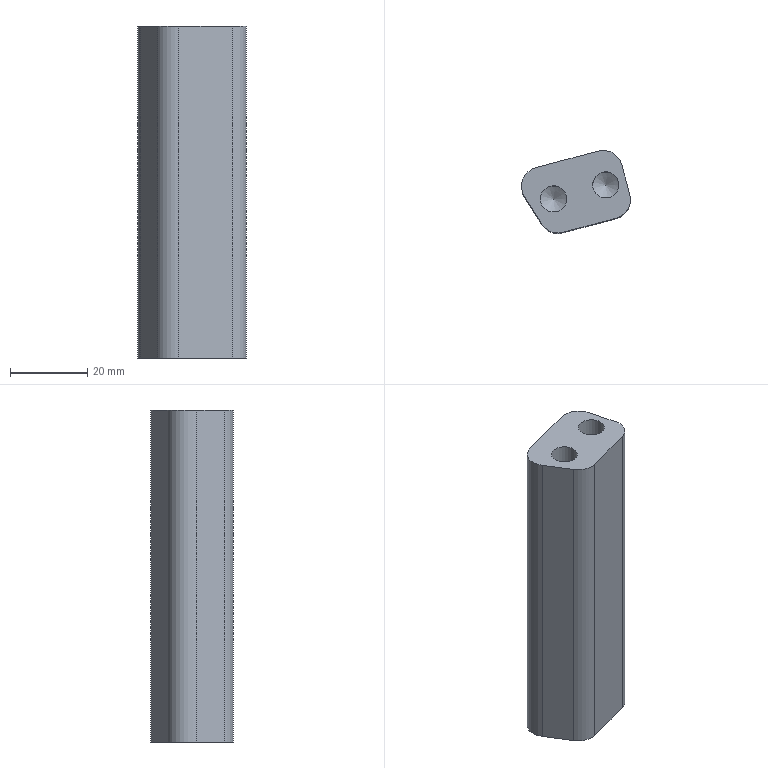Part | NX | features solid 2 | 1 solid | 14 faces | box 28.217 x 21.421 x 86 mm | volume 35584 mm3 | cylinder 6 | plane 6 | cone 2 | commonest cylinder face diameters 10 x4 6.8 x2
STEP:
#1=CARTESIAN_POINT('',(1387.735,54.431,48.508));
#2=VERTEX_POINT('',#1);
#3=CARTESIAN_POINT('',(1384.335,54.431,48.508));
#4=DIRECTION('',(0.,0.,-1.));
#5=DIRECTION('',(1.,0.,0.));
#6=AXIS2_PLACEMENT_3D('',#3,#4,#5);
#7=CIRCLE('',#6,3.4);
#8=EDGE_CURVE('',#2,#2,#7,.F.);
#9=ORIENTED_EDGE('',*,*,#8,.T.);
#10=EDGE_LOOP('',(#9));
#11=FACE_BOUND('',#10,.T.);
#12=CARTESIAN_POINT('',(1384.335,54.431,46.465));
#13=VERTEX_POINT('',#12);
#14=VERTEX_LOOP('',#13);
#15=FACE_BOUND('',#14,.T.);
#16=CARTESIAN_POINT('',(1384.335,54.431,49.018));
#17=DIRECTION('',(0.,0.,1.));
#18=DIRECTION('',(1.,0.,0.));
#19=AXIS2_PLACEMENT_3D('',#16,#17,#18);
#20=CONICAL_SURFACE('',#19,4.25,1.03);
#21=ADVANCED_FACE('',(#11,#15),#20,.F.);
#22=ORIENTED_EDGE('',*,*,#8,.F.);
#23=EDGE_LOOP('',(#22));
#24=FACE_BOUND('',#23,.T.);
#25=CARTESIAN_POINT('',(1380.935,54.431,78.));
#26=VERTEX_POINT('',#25);
#27=CARTESIAN_POINT('',(1384.335,54.431,78.));
#28=DIRECTION('',(0.,0.,1.));
#29=DIRECTION('',(-1.,0.,0.));
#30=AXIS2_PLACEMENT_3D('',#27,#28,#29);
#31=CIRCLE('',#30,3.4);
#32=EDGE_CURVE('',#26,#26,#31,.T.);
#33=ORIENTED_EDGE('',*,*,#32,.T.);
#34=EDGE_LOOP('',(#33));
#35=FACE_BOUND('',#34,.T.);
#36=CARTESIAN_POINT('',(1384.335,54.431,79.018));
#37=DIRECTION('',(0.,0.,-1.));
#38=DIRECTION('',(-1.,0.,0.));
#39=AXIS2_PLACEMENT_3D('',#36,#37,#38);
#40=CYLINDRICAL_SURFACE('',#39,3.4);
#41=ADVANCED_FACE('',(#24,#35),#40,.F.);
#42=CARTESIAN_POINT('',(1366.205,58.89,-8.));
#43=VERTEX_POINT('',#42);
#44=CARTESIAN_POINT('',(1382.352,63.217,-8.));
#45=VERTEX_POINT('',#44);
#46=CARTESIAN_POINT('',(1366.205,58.89,-8.));
#47=DIRECTION('',(0.9659,0.2588,0.));
#48=VECTOR('',#47,1000.);
#49=LINE('',#46,#48);
#50=EDGE_CURVE('',#43,#45,#49,.T.);
#51=ORIENTED_EDGE('',*,*,#50,.T.);
#52=CARTESIAN_POINT('',(1388.475,59.681,-8.));
#53=VERTEX_POINT('',#52);
#54=CARTESIAN_POINT('',(1383.646,58.387,-8.));
#55=DIRECTION('',(0.,0.,-1.));
#56=DIRECTION('',(-1.,0.,0.));
#57=AXIS2_PLACEMENT_3D('',#54,#55,#56);
#58=CIRCLE('',#57,5.);
#59=EDGE_CURVE('',#45,#53,#58,.T.);
#60=ORIENTED_EDGE('',*,*,#59,.T.);
#61=CARTESIAN_POINT('',(1390.546,51.954,-8.));
#62=VERTEX_POINT('',#61);
#63=CARTESIAN_POINT('',(1388.475,59.681,-8.));
#64=DIRECTION('',(0.2588,-0.9659,0.));
#65=VECTOR('',#64,1000.);
#66=LINE('',#63,#65);
#67=EDGE_CURVE('',#53,#62,#66,.T.);
#68=ORIENTED_EDGE('',*,*,#67,.T.);
#69=CARTESIAN_POINT('',(1387.01,45.83,-8.));
#70=VERTEX_POINT('',#69);
#71=CARTESIAN_POINT('',(1385.716,50.66,-8.));
#72=DIRECTION('',(0.,0.,-1.));
#73=DIRECTION('',(-1.,0.,0.));
#74=AXIS2_PLACEMENT_3D('',#71,#72,#73);
#75=CIRCLE('',#74,5.);
#76=EDGE_CURVE('',#62,#70,#75,.T.);
#77=ORIENTED_EDGE('',*,*,#76,.T.);
#78=CARTESIAN_POINT('',(1373.226,42.137,-8.));
#79=VERTEX_POINT('',#78);
#80=CARTESIAN_POINT('',(1387.01,45.83,-8.));
#81=DIRECTION('',(-0.9659,-0.2588,0.));
#82=VECTOR('',#81,1000.);
#83=LINE('',#80,#82);
#84=EDGE_CURVE('',#70,#79,#83,.T.);
#85=ORIENTED_EDGE('',*,*,#84,.T.);
#86=CARTESIAN_POINT('',(1367.692,44.317,-8.));
#87=VERTEX_POINT('',#86);
#88=CARTESIAN_POINT('',(1371.932,46.966,-8.));
#89=DIRECTION('',(0.,0.,-1.));
#90=DIRECTION('',(-1.,0.,0.));
#91=AXIS2_PLACEMENT_3D('',#88,#89,#90);
#92=CIRCLE('',#91,5.);
#93=EDGE_CURVE('',#79,#87,#92,.T.);
#94=ORIENTED_EDGE('',*,*,#93,.T.);
#95=CARTESIAN_POINT('',(1363.259,51.411,-8.));
#96=VERTEX_POINT('',#95);
#97=CARTESIAN_POINT('',(1367.692,44.317,-8.));
#98=DIRECTION('',(-0.5299,0.848,0.));
#99=VECTOR('',#98,1000.);
#100=LINE('',#97,#99);
#101=EDGE_CURVE('',#87,#96,#100,.T.);
#102=ORIENTED_EDGE('',*,*,#101,.T.);
#103=CARTESIAN_POINT('',(1367.499,54.061,-8.));
#104=DIRECTION('',(0.,0.,-1.));
#105=DIRECTION('',(-1.,0.,0.));
#106=AXIS2_PLACEMENT_3D('',#103,#104,#105);
#107=CIRCLE('',#106,5.);
#108=EDGE_CURVE('',#96,#43,#107,.T.);
#109=ORIENTED_EDGE('',*,*,#108,.T.);
#110=EDGE_LOOP('',(#51,#60,#68,#77,#85,#94,#102,#109));
#111=FACE_BOUND('',#110,.T.);
#112=CARTESIAN_POINT('',(1383.646,58.387,-8.));
#113=DIRECTION('',(0.,0.,-1.));
#114=DIRECTION('',(-1.,0.,0.));
#115=AXIS2_PLACEMENT_3D('',#112,#113,#114);
#116=PLANE('',#115);
#117=ADVANCED_FACE('',(#111),#116,.T.);
#118=CARTESIAN_POINT('',(1374.212,50.807,48.508));
#119=VERTEX_POINT('',#118);
#120=CARTESIAN_POINT('',(1370.812,50.807,48.508));
#121=DIRECTION('',(0.,0.,-1.));
#122=DIRECTION('',(1.,0.,0.));
#123=AXIS2_PLACEMENT_3D('',#120,#121,#122);
#124=CIRCLE('',#123,3.4);
#125=EDGE_CURVE('',#119,#119,#124,.F.);
#126=ORIENTED_EDGE('',*,*,#125,.T.);
#127=EDGE_LOOP('',(#126));
#128=FACE_BOUND('',#127,.T.);
#129=CARTESIAN_POINT('',(1370.812,50.807,46.465));
#130=VERTEX_POINT('',#129);
#131=VERTEX_LOOP('',#130);
#132=FACE_BOUND('',#131,.T.);
#133=CARTESIAN_POINT('',(1370.812,50.807,49.018));
#134=DIRECTION('',(0.,0.,1.));
#135=DIRECTION('',(1.,0.,0.));
#136=AXIS2_PLACEMENT_3D('',#133,#134,#135);
#137=CONICAL_SURFACE('',#136,4.25,1.03);
#138=ADVANCED_FACE('',(#128,#132),#137,.F.);
#139=ORIENTED_EDGE('',*,*,#108,.F.);
#140=CARTESIAN_POINT('',(1363.259,51.411,78.));
#141=VERTEX_POINT('',#140);
#142=CARTESIAN_POINT('',(1363.259,51.411,82.));
#143=DIRECTION('',(0.,0.,-1.));
#144=VECTOR('',#143,1000.);
#145=LINE('',#142,#144);
#146=EDGE_CURVE('',#141,#96,#145,.T.);
#147=ORIENTED_EDGE('',*,*,#146,.F.);
#148=CARTESIAN_POINT('',(1366.205,58.89,78.));
#149=VERTEX_POINT('',#148);
#150=CARTESIAN_POINT('',(1367.499,54.061,78.));
#151=DIRECTION('',(0.,0.,-1.));
#152=DIRECTION('',(-1.,0.,0.));
#153=AXIS2_PLACEMENT_3D('',#150,#151,#152);
#154=CIRCLE('',#153,5.);
#155=EDGE_CURVE('',#141,#149,#154,.T.);
#156=ORIENTED_EDGE('',*,*,#155,.T.);
#157=CARTESIAN_POINT('',(1366.205,58.89,82.));
#158=DIRECTION('',(0.,0.,-1.));
#159=VECTOR('',#158,1000.);
#160=LINE('',#157,#159);
#161=EDGE_CURVE('',#149,#43,#160,.T.);
#162=ORIENTED_EDGE('',*,*,#161,.T.);
#163=EDGE_LOOP('',(#139,#147,#156,#162));
#164=FACE_BOUND('',#163,.T.);
#165=CARTESIAN_POINT('',(1367.499,54.061,82.));
#166=DIRECTION('',(0.,0.,-1.));
#167=DIRECTION('',(-1.,0.,0.));
#168=AXIS2_PLACEMENT_3D('',#165,#166,#167);
#169=CYLINDRICAL_SURFACE('',#168,5.);
#170=ADVANCED_FACE('',(#164),#169,.T.);
#171=ORIENTED_EDGE('',*,*,#101,.F.);
#172=CARTESIAN_POINT('',(1367.692,44.317,78.));
#173=VERTEX_POINT('',#172);
#174=CARTESIAN_POINT('',(1367.692,44.317,82.));
#175=DIRECTION('',(0.,0.,-1.));
#176=VECTOR('',#175,1000.);
#177=LINE('',#174,#176);
#178=EDGE_CURVE('',#173,#87,#177,.T.);
#179=ORIENTED_EDGE('',*,*,#178,.F.);
#180=CARTESIAN_POINT('',(1589.644,-310.881,78.));
#181=DIRECTION('',(-0.5299,0.848,0.));
#182=VECTOR('',#181,1000.);
#183=LINE('',#180,#182);
#184=EDGE_CURVE('',#173,#141,#183,.T.);
#185=ORIENTED_EDGE('',*,*,#184,.T.);
#186=ORIENTED_EDGE('',*,*,#146,.T.);
#187=EDGE_LOOP('',(#171,#179,#185,#186));
#188=FACE_BOUND('',#187,.T.);
#189=CARTESIAN_POINT('',(1367.692,44.317,82.));
#190=DIRECTION('',(-0.848,-0.5299,0.));
#191=DIRECTION('',(0.5299,-0.848,0.));
#192=AXIS2_PLACEMENT_3D('',#189,#190,#191);
#193=PLANE('',#192);
#194=ADVANCED_FACE('',(#188),#193,.T.);
#195=ORIENTED_EDGE('',*,*,#93,.F.);
#196=CARTESIAN_POINT('',(1373.226,42.137,78.));
#197=VERTEX_POINT('',#196);
#198=CARTESIAN_POINT('',(1373.226,42.137,82.));
#199=DIRECTION('',(0.,0.,-1.));
#200=VECTOR('',#199,1000.);
#201=LINE('',#198,#200);
#202=EDGE_CURVE('',#197,#79,#201,.T.);
#203=ORIENTED_EDGE('',*,*,#202,.F.);
#204=CARTESIAN_POINT('',(1371.932,46.966,78.));
#205=DIRECTION('',(0.,0.,-1.));
#206=DIRECTION('',(-1.,0.,0.));
#207=AXIS2_PLACEMENT_3D('',#204,#205,#206);
#208=CIRCLE('',#207,5.);
#209=EDGE_CURVE('',#197,#173,#208,.T.);
#210=ORIENTED_EDGE('',*,*,#209,.T.);
#211=ORIENTED_EDGE('',*,*,#178,.T.);
#212=EDGE_LOOP('',(#195,#203,#210,#211));
#213=FACE_BOUND('',#212,.T.);
#214=CARTESIAN_POINT('',(1371.932,46.966,82.));
#215=DIRECTION('',(0.,0.,-1.));
#216=DIRECTION('',(-1.,0.,0.));
#217=AXIS2_PLACEMENT_3D('',#214,#215,#216);
#218=CYLINDRICAL_SURFACE('',#217,5.);
#219=ADVANCED_FACE('',(#213),#218,.T.);
#220=ORIENTED_EDGE('',*,*,#84,.F.);
#221=CARTESIAN_POINT('',(1387.01,45.83,78.));
#222=VERTEX_POINT('',#221);
#223=CARTESIAN_POINT('',(1387.01,45.83,82.));
#224=DIRECTION('',(0.,0.,-1.));
#225=VECTOR('',#224,1000.);
#226=LINE('',#223,#225);
#227=EDGE_CURVE('',#222,#70,#226,.T.);
#228=ORIENTED_EDGE('',*,*,#227,.F.);
#229=CARTESIAN_POINT('',(2028.799,217.797,78.));
#230=DIRECTION('',(-0.9659,-0.2588,0.));
#231=VECTOR('',#230,1000.);
#232=LINE('',#229,#231);
#233=EDGE_CURVE('',#222,#197,#232,.T.);
#234=ORIENTED_EDGE('',*,*,#233,.T.);
#235=ORIENTED_EDGE('',*,*,#202,.T.);
#236=EDGE_LOOP('',(#220,#228,#234,#235));
#237=FACE_BOUND('',#236,.T.);
#238=CARTESIAN_POINT('',(1387.01,45.83,82.));
#239=DIRECTION('',(0.2588,-0.9659,0.));
#240=DIRECTION('',(0.9659,0.2588,0.));
#241=AXIS2_PLACEMENT_3D('',#238,#239,#240);
#242=PLANE('',#241);
#243=ADVANCED_FACE('',(#237),#242,.T.);
#244=ORIENTED_EDGE('',*,*,#76,.F.);
#245=CARTESIAN_POINT('',(1390.546,51.954,78.));
#246=VERTEX_POINT('',#245);
#247=CARTESIAN_POINT('',(1390.546,51.954,82.));
#248=DIRECTION('',(0.,0.,-1.));
#249=VECTOR('',#248,1000.);
#250=LINE('',#247,#249);
#251=EDGE_CURVE('',#246,#62,#250,.T.);
#252=ORIENTED_EDGE('',*,*,#251,.F.);
#253=CARTESIAN_POINT('',(1385.716,50.66,78.));
#254=DIRECTION('',(0.,0.,-1.));
#255=DIRECTION('',(-1.,0.,0.));
#256=AXIS2_PLACEMENT_3D('',#253,#254,#255);
#257=CIRCLE('',#256,5.);
#258=EDGE_CURVE('',#246,#222,#257,.T.);
#259=ORIENTED_EDGE('',*,*,#258,.T.);
#260=ORIENTED_EDGE('',*,*,#227,.T.);
#261=EDGE_LOOP('',(#244,#252,#259,#260));
#262=FACE_BOUND('',#261,.T.);
#263=CARTESIAN_POINT('',(1385.716,50.66,82.));
#264=DIRECTION('',(0.,0.,-1.));
#265=DIRECTION('',(-1.,0.,0.));
#266=AXIS2_PLACEMENT_3D('',#263,#264,#265);
#267=CYLINDRICAL_SURFACE('',#266,5.);
#268=ADVANCED_FACE('',(#262),#267,.T.);
#269=ORIENTED_EDGE('',*,*,#67,.F.);
#270=CARTESIAN_POINT('',(1388.475,59.681,78.));
#271=VERTEX_POINT('',#270);
#272=CARTESIAN_POINT('',(1388.475,59.681,82.));
#273=DIRECTION('',(0.,0.,-1.));
#274=VECTOR('',#273,1000.);
#275=LINE('',#272,#274);
#276=EDGE_CURVE('',#271,#53,#275,.T.);
#277=ORIENTED_EDGE('',*,*,#276,.F.);
#278=CARTESIAN_POINT('',(1450.198,-170.673,78.));
#279=DIRECTION('',(0.2588,-0.9659,0.));
#280=VECTOR('',#279,1000.);
#281=LINE('',#278,#280);
#282=EDGE_CURVE('',#271,#246,#281,.T.);
#283=ORIENTED_EDGE('',*,*,#282,.T.);
#284=ORIENTED_EDGE('',*,*,#251,.T.);
#285=EDGE_LOOP('',(#269,#277,#283,#284));
#286=FACE_BOUND('',#285,.T.);
#287=CARTESIAN_POINT('',(1388.475,59.681,82.));
#288=DIRECTION('',(0.9659,0.2588,0.));
#289=DIRECTION('',(-0.2588,0.9659,0.));
#290=AXIS2_PLACEMENT_3D('',#287,#288,#289);
#291=PLANE('',#290);
#292=ADVANCED_FACE('',(#286),#291,.T.);
#293=ORIENTED_EDGE('',*,*,#59,.F.);
#294=CARTESIAN_POINT('',(1382.352,63.217,78.));
#295=VERTEX_POINT('',#294);
#296=CARTESIAN_POINT('',(1382.352,63.217,82.));
#297=DIRECTION('',(0.,0.,-1.));
#298=VECTOR('',#297,1000.);
#299=LINE('',#296,#298);
#300=EDGE_CURVE('',#295,#45,#299,.T.);
#301=ORIENTED_EDGE('',*,*,#300,.F.);
#302=CARTESIAN_POINT('',(1383.646,58.387,78.));
#303=DIRECTION('',(0.,0.,-1.));
#304=DIRECTION('',(-1.,0.,0.));
#305=AXIS2_PLACEMENT_3D('',#302,#303,#304);
#306=CIRCLE('',#305,5.);
#307=EDGE_CURVE('',#295,#271,#306,.T.);
#308=ORIENTED_EDGE('',*,*,#307,.T.);
#309=ORIENTED_EDGE('',*,*,#276,.T.);
#310=EDGE_LOOP('',(#293,#301,#308,#309));
#311=FACE_BOUND('',#310,.T.);
#312=CARTESIAN_POINT('',(1383.646,58.387,82.));
#313=DIRECTION('',(0.,0.,-1.));
#314=DIRECTION('',(-1.,0.,0.));
#315=AXIS2_PLACEMENT_3D('',#312,#313,#314);
#316=CYLINDRICAL_SURFACE('',#315,5.);
#317=ADVANCED_FACE('',(#311),#316,.T.);
#318=ORIENTED_EDGE('',*,*,#50,.F.);
#319=ORIENTED_EDGE('',*,*,#161,.F.);
#320=CARTESIAN_POINT('',(2024.14,235.184,78.));
#321=DIRECTION('',(0.9659,0.2588,0.));
#322=VECTOR('',#321,1000.);
#323=LINE('',#320,#322);
#324=EDGE_CURVE('',#149,#295,#323,.T.);
#325=ORIENTED_EDGE('',*,*,#324,.T.);
#326=ORIENTED_EDGE('',*,*,#300,.T.);
#327=EDGE_LOOP('',(#318,#319,#325,#326));
#328=FACE_BOUND('',#327,.T.);
#329=CARTESIAN_POINT('',(1366.205,58.89,82.));
#330=DIRECTION('',(-0.2588,0.9659,0.));
#331=DIRECTION('',(-0.9659,-0.2588,0.));
#332=AXIS2_PLACEMENT_3D('',#329,#330,#331);
#333=PLANE('',#332);
#334=ADVANCED_FACE('',(#328),#333,.T.);
#335=ORIENTED_EDGE('',*,*,#125,.F.);
#336=EDGE_LOOP('',(#335));
#337=FACE_BOUND('',#336,.T.);
#338=CARTESIAN_POINT('',(1367.412,50.807,78.));
#339=VERTEX_POINT('',#338);
#340=CARTESIAN_POINT('',(1370.812,50.807,78.));
#341=DIRECTION('',(0.,0.,1.));
#342=DIRECTION('',(-1.,0.,0.));
#343=AXIS2_PLACEMENT_3D('',#340,#341,#342);
#344=CIRCLE('',#343,3.4);
#345=EDGE_CURVE('',#339,#339,#344,.F.);
#346=ORIENTED_EDGE('',*,*,#345,.F.);
#347=EDGE_LOOP('',(#346));
#348=FACE_BOUND('',#347,.T.);
#349=CARTESIAN_POINT('',(1370.812,50.807,79.018));
#350=DIRECTION('',(0.,0.,-1.));
#351=DIRECTION('',(-1.,0.,0.));
#352=AXIS2_PLACEMENT_3D('',#349,#350,#351);
#353=CYLINDRICAL_SURFACE('',#352,3.4);
#354=ADVANCED_FACE('',(#337,#348),#353,.F.);
#355=ORIENTED_EDGE('',*,*,#32,.F.);
#356=EDGE_LOOP('',(#355));
#357=FACE_BOUND('',#356,.T.);
#358=ORIENTED_EDGE('',*,*,#345,.T.);
#359=EDGE_LOOP('',(#358));
#360=FACE_BOUND('',#359,.T.);
#361=ORIENTED_EDGE('',*,*,#324,.F.);
#362=ORIENTED_EDGE('',*,*,#155,.F.);
#363=ORIENTED_EDGE('',*,*,#184,.F.);
#364=ORIENTED_EDGE('',*,*,#209,.F.);
#365=ORIENTED_EDGE('',*,*,#233,.F.);
#366=ORIENTED_EDGE('',*,*,#258,.F.);
#367=ORIENTED_EDGE('',*,*,#282,.F.);
#368=ORIENTED_EDGE('',*,*,#307,.F.);
#369=EDGE_LOOP('',(#361,#362,#363,#364,#365,#366,#367,#368));
#370=FACE_BOUND('',#369,.T.);
#371=CARTESIAN_POINT('',(2087.158,0.000000688,78.));
#372=DIRECTION('',(0.,0.,-1.));
#373=DIRECTION('',(1.,0.,0.));
#374=AXIS2_PLACEMENT_3D('',#371,#372,#373);
#375=PLANE('',#374);
#376=ADVANCED_FACE('',(#357,#360,#370),#375,.F.);
#377=CLOSED_SHELL('',(#21,#41,#117,#138,#170,#194,#219,#243,#268,#292,#317,#334,#354,#376));
#378=MANIFOLD_SOLID_BREP('',#377);
#379=(LENGTH_UNIT()NAMED_UNIT(*)SI_UNIT(.MILLI.,.METRE.));
#380=UNCERTAINTY_MEASURE_WITH_UNIT(LENGTH_MEASURE(0.00001),#379,'','');
#381=(NAMED_UNIT(*)PLANE_ANGLE_UNIT()SI_UNIT($,.RADIAN.));
#382=(NAMED_UNIT(*)SI_UNIT($,.STERADIAN.)SOLID_ANGLE_UNIT());
#383=(GEOMETRIC_REPRESENTATION_CONTEXT(3)GLOBAL_UNCERTAINTY_ASSIGNED_CONTEXT((#380))GLOBAL_UNIT_ASSIGNED_CONTEXT((#379,#381,#382))REPRESENTATION_CONTEXT('',''));
#384=ADVANCED_BREP_SHAPE_REPRESENTATION('',(#378),#383);